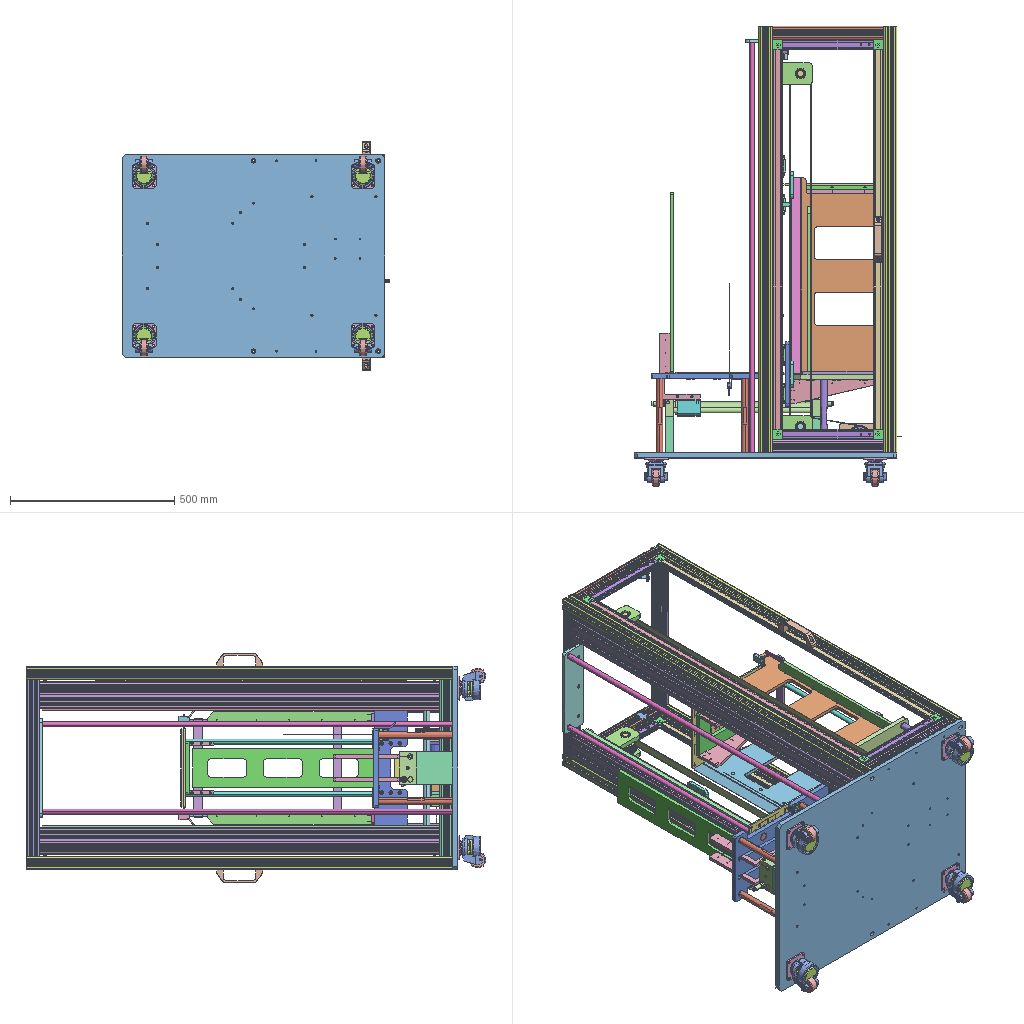Assembly | STEP file | 78 different items | 208 placed | box 815 x 1400 x 700 mm
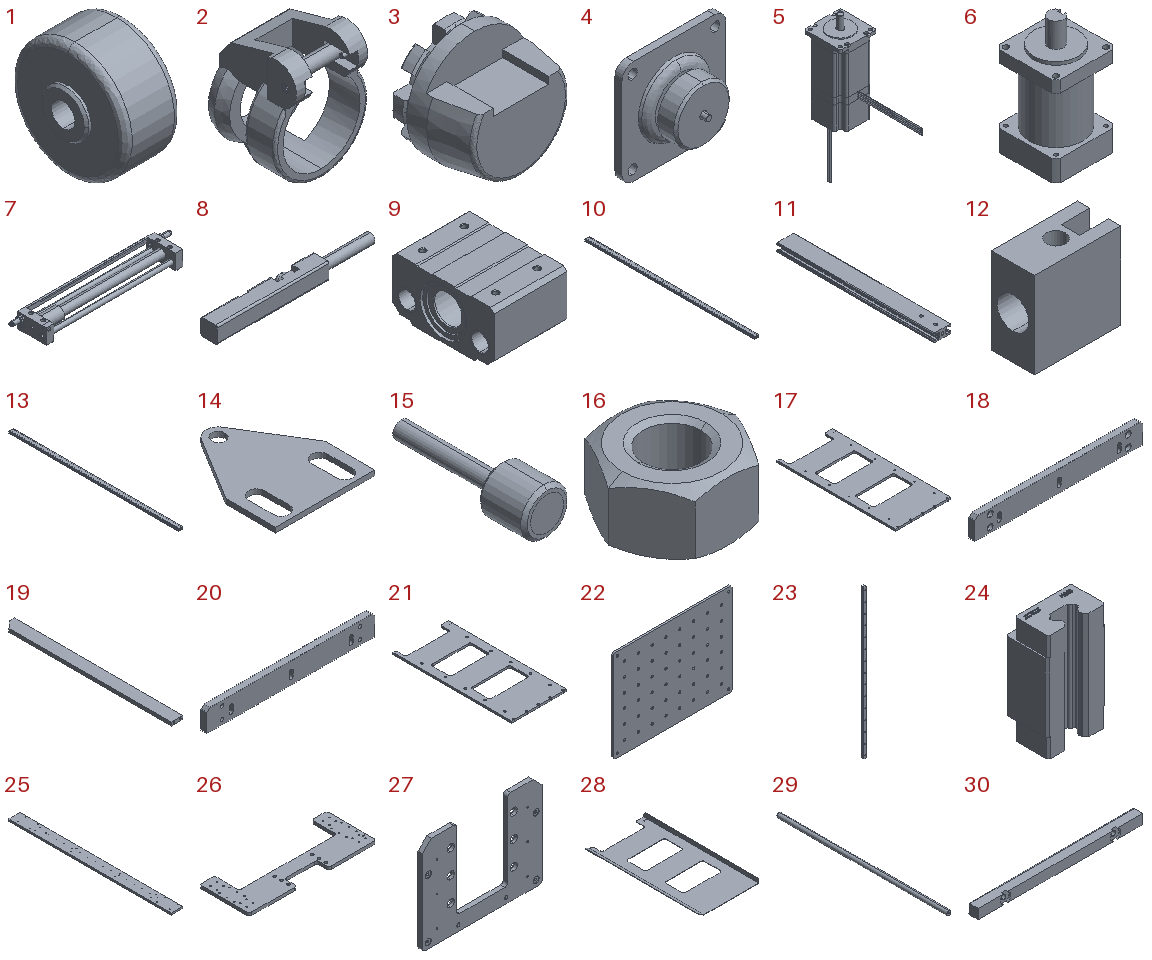Parts list (item | name | quantity | parent item | size | volume):
1 | HI_CGR51-60-U-001 | x4 | in CGR51-60-U, CGR51-60-U-1, CGR51-60-U-2, CGR51-60-U-3 | 28 x 49 x 49 mm | 43678 mm3
2 | HI_CGR51-60-U-002 | x4 | in CGR51-60-U, CGR51-60-U-1, CGR51-60-U-2, CGR51-60-U-3 | 70 x 63 x 89.5 mm | 81661 mm3
3 | HI_CGR51-60-U-004 | x4 | in CGR51-60-U, CGR51-60-U-1, CGR51-60-U-2, CGR51-60-U-3 | 55 x 39.5 x 55 mm | 65698 mm3
4 | HI_CGR51-60-U-003 | x4 | in CGR51-60-U, CGR51-60-U-1, CGR51-60-U-2, CGR51-60-U-3 | 73 x 29.8 x 73 mm | 47628 mm3
5 | Leadshine 57HSB21A (with brake) | x1 | in 57 Leadshine stepper with brake and 2-stage reducer (1:30) assembly | 57.15 x 157.15 x 237 mm | 340795 mm3
6 | 57 stepper reducer, 2-stage, ratio 30 | x1 | in 57 Leadshine stepper with brake and 2-stage reducer (1:30) assembly | 57 x 57 x 110 mm | 202914 mm3
7 | _RMT-25X350-S-A(0)-GN-2_rod | x1 | in RMT25X350SA_0_+_DS1-GN-2_ | 555 x 106.4 x 53 mm | 757073 mm3
8 | _CS1-E | x2 | in RMT25X350SA_0_+_DS1-GN-2_ | 48.8 x 5.2 x 5 mm | 895.745 mm3
9 | _RMT-25X350-S(0)_body | x1 | in RMT25X350SA_0_+_DS1-GN-2_ | 70 x 97 x 52 mm | 215787 mm3
10 | GB1530T-6-30x15x1155-BASHOU | x2 | in 1220x340 door, 1220x340 door-1 | 30 x 1157 x 15 mm | 281206 mm3
11 | GB1530T-6-30x15x275 | x4 | in 1220x340 door, 1220x340 door-1 | 30 x 277 x 15 mm | 67010 mm3
12 | Right-angle connecting block | x8 | in 1220x340 door, 1220x340 door-1 | 30 x 15 x 30 mm | 8895 mm3
13 | GB1530T-6-30x15x1155 | x2 | in 1220x340 door, 1220x340 door-1 | 30 x 1157 x 15 mm | 281619 mm3
14 | Door catch sheet metal | x4 | in Door catch, Door catch-1, Door catch-2, Door catch-3 | 40 x 48 x 2 mm | 2431 mm3
15 | Pedestal magnet | x4 | in Door catch, Door catch-1, Door catch-2, Door catch-3 | 14 x 44 x 14 mm | 2702 mm3
16 | hex nuts, style 1-grades ab gb(GB_FASTENER_NUT_SNAB1 M5-N) | x8 | in Door catch, Door catch-1, Door catch-2, Door catch-3 | 9.238 x 8 x 4.7 mm | 190.603 mm3
17 | PN_0033 | x1 | in Side bracket | 279.996 x 599.997 x 10 mm | 1160926 mm3
18 | PN_0034 | x1 | in Side bracket | 280 x 10 x 35 mm | 92081 mm3
19 | PN_0035 | x4 | in Side bracket | 35 x 500 x 10 mm | 171757 mm3
20 | PN_0037 | x1 | in Side bracket | 280 x 10 x 35 mm | 92081 mm3
21 | PN_0036 | x1 | in Side bracket | 279.996 x 599.997 x 10 mm | 1160926 mm3
22 | Three-part square aluminium plate (2R8, 6R5) | x3 | - | 310 x 4.5 x 240 mm | 298192 mm3
23 | HGR15-rail L870 | x2 | - | 15 x 15 x 870 mm | 160134 mm3
24 | HGH15-slider | x8 | - | 34 x 23.7 x 61.7 mm | 37046 mm3
25 | PN_0029 | x1 | - | 90 x 1255 x 15 mm | 1602482 mm3
26 | PN_0002 | x1 | - | 510 x 200 x 12 mm | 664330 mm3
27 | PN_0003 | x1 | - | 400 x 15 x 315 mm | 1138040 mm3
28 | PN_0004(Default) | x1 | - | 313.731 x 597.76 x 21.5 mm | 225169 mm3
29 | PN_0005 | x2 | - | 15 x 580 x 15 mm | 101796 mm3
30 | PN_0006 | x1 | - | 240 x 15 x 14 mm | 46724 mm3
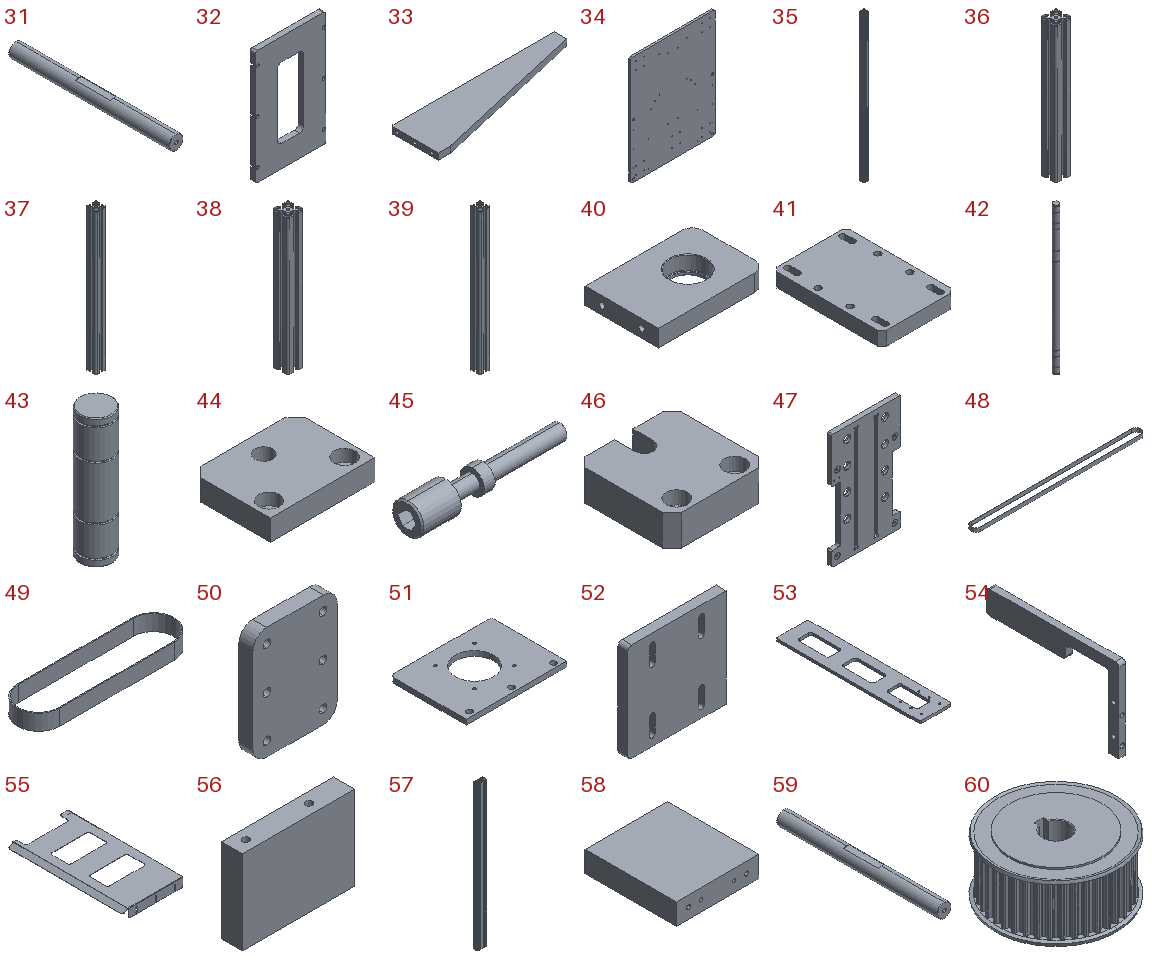31 | PN_0007 | x4 | - | 20 x 228 x 20 mm | 70235 mm3
32 | PN_0008 | x2 | - | 160 x 12 x 260 mm | 379891 mm3
33 | PN_0009 | x4 | - | 260 x 75 x 10 mm | 127129 mm3
34 | PN_0010 | x1 | - | 620 x 15 x 800 mm | 7409131 mm3
35 | HM-8-4040D-L1300 | x4 | - | 40 x 40 x 1300 mm | 890054 mm3
36 | HM-8-4040D-L340-machining required | x2 | - | 40 x 40 x 340 mm | 231664 mm3
37 | HM-8-4040D-L540-machining required | x1 | - | 40 x 40 x 540 mm | 368969 mm3
38 | HM-8-4040D-L340 | x2 | - | 40 x 40 x 340 mm | 232783 mm3
39 | HM-8-4040D-L540 | x2 | - | 40 x 40 x 540 mm | 369715 mm3
40 | PN_0012 | x8 | - | 95 x 65 x 15 mm | 79674 mm3
41 | PN_0013 | x4 | - | 80 x 120 x 15 mm | 132965 mm3
42 | PN_0014 | x1 | - | 20 x 20 x 530 mm | 164764 mm3
43 | PN_0015 | x2 | - | 20 x 20 x 80 mm | 24503 mm3
44 | PN_0016 | x2 | - | 50 x 38 x 10 mm | 17083 mm3
45 | AJKTN10-50 adjusting screw | x2 | - | 99 x 20 x 20 mm | 13265 mm3
46 | PN_0017 | x2 | - | 50 x 50 x 16 mm | 35086 mm3
47 | PN_0018 | x1 | - | 240 x 15 x 400 mm | 1068440 mm3
48 | Timing belt S5M-width 25-length 2350 (C-HTBN2350S5M-250, steel wire core) | x2 | - | 1142 x 66.7 x 25 mm | 88306 mm3
49 | Timing belt S5M-width 25-length 565 (steel wire core) | x1 | - | 249.2 x 66.7 x 25 mm | 21369 mm3
50 | PN_0021 | x4 | - | 60 x 10 x 80 mm | 43843 mm3
51 | PN_0022 | x1 | - | 120 x 90 x 6 mm | 54372 mm3
52 | PN_0023 | x1 | - | 120 x 12 x 120 mm | 163808 mm3
53 | PN_0011 | x1 | - | 120 x 550 x 10 mm | 459826 mm3
54 | PN_0019 | x2 | - | 10 x 200 x 125 mm | 67703 mm3
55 | PN_0024(Default) | x1 | - | 313.731 x 599.997 x 46.5 mm | 244261 mm3
56 | PN_0025 | x1 | - | 80 x 15 x 60 mm | 69644 mm3
57 | HM-8-4080D-L1220 | x2 | - | 80 x 40 x 1220 mm | 1475152 mm3
58 | PN_0020 | x2 | - | 100 x 110 x 25.5 mm | 279122 mm3
59 | PN_0026 | x4 | - | 20 x 230 x 20 mm | 70863 mm3
60 | EBJ52-S5M250-40-A-N-d14 | x1 | - | 67 x 67 x 32 mm | 87087 mm3
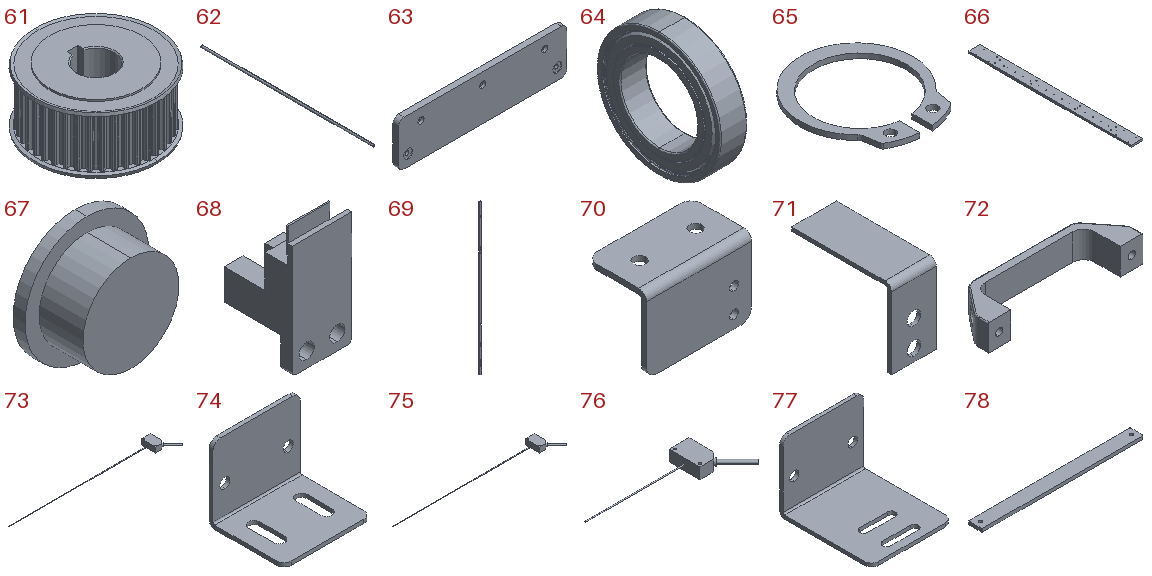61 | EBJ52-S5M250-40-A-N-d20 | x5 | - | 67 x 67 x 32 mm | 81650 mm3
62 | PN_0027 | x2 | - | 16 x 1252 x 16 mm | 251030 mm3
63 | PN_0028 | x1 | - | 300 x 10 x 80 mm | 235858 mm3
64 | BAY6804ZZ lifting mechanism drive bearing | x8 | - | 7 x 32 x 32 mm | 2847 mm3
65 | Shaft retaining ring 20 (GB_CONNECTING_PIECE_RING_RRA 20) | x8 | - | 22.5 x 25.161 x 1 mm | 153.893 mm3
66 | PN_0001 | x1 | - | 90 x 1255 x 15 mm | 1602655 mm3
67 | Universal ball bearing H21xD31xh6-40KG | x14 | - | 31 x 21 x 31 mm | 8224 mm3
68 | xgSENSOR(EE-SX674) | x4 | - | 13.6 x 15.5 x 27.3 mm | 2060 mm3
69 | 9x6 sensor aluminium slot M3 type-L950 | x1 | - | 9 x 6 x 950 mm | 30935 mm3
70 | PN_0030(Default) | x4 | - | 30 x 17.237 x 21.5 mm | 1592 mm3
71 | PN_0031(Default) | x1 | - | 12 x 26.737 x 21 mm | 534.113 mm3
72 | Door handle | x2 | - | 140 x 40 x 24 mm | 37832 mm3
73 | Photoelectric sensor CX421 (NPN, 300mm) | x1 | - | 341.148 x 54.448 x 11.2 mm | 7391 mm3
74 | PN_0038(Default) | x1 | - | 35 x 30 x 30 mm | 2806 mm3
75 | Photoelectric sensor CX411D (NPN, receiver, with slit light shield OS-CX-2)) | x1 | - | 341.148 x 54.448 x 11.2 mm | 7391 mm3
76 | Photoelectric sensor CX411D (NPN, receiver) | x1 | - | 141.148 x 54.448 x 11.2 mm | 7234 mm3
77 | PN_0039(Default) | x2 | - | 35 x 40 x 30 mm | 3359 mm3
78 | PN_0032 | x2 | - | 300 x 25 x 6 mm | 44703 mm3
Placements (level | parent | child | x y z in mm | rotation matrix by rows):
1 | subassembly 2 | CGR51-60-U | -198.5 -701.0 280.0 | 1 0 0 0 1 0 0 0 1
2 | CGR51-60-U | HI_CGR51-60-U-001 | -0.0 -0.0 -0.0 | 1 0 0 0 1 0 0 0 1
2 | CGR51-60-U | HI_CGR51-60-U-002 | -0.0 -0.0 -0.0 | 1 0 0 0 1 0 0 0 1
2 | CGR51-60-U | HI_CGR51-60-U-004 | -0.0 -0.0 -0.0 | 1 0 0 0 1 0 0 0 1
2 | CGR51-60-U | HI_CGR51-60-U-003 | -0.0 4.0 -0.0 | 1 0 0 0 1 0 0 0 1
1 | subassembly 2 | CGR51-60-U-1 | -198.5 -701.0 -280.0 | -1 0 0 0 1 0 0 0 -1
2 | CGR51-60-U-1 | HI_CGR51-60-U-001 | -0.0 -0.0 -0.0 | 1 0 0 0 1 0 0 0 1
2 | CGR51-60-U-1 | HI_CGR51-60-U-002 | -0.0 -0.0 -0.0 | 1 0 0 0 1 0 0 0 1
2 | CGR51-60-U-1 | HI_CGR51-60-U-004 | -0.0 -0.0 -0.0 | 1 0 0 0 1 0 0 0 1
2 | CGR51-60-U-1 | HI_CGR51-60-U-003 | -0.0 4.0 -0.0 | 1 0 0 0 1 0 0 0 1
1 | subassembly 2 | CGR51-60-U-2 | 468.5 -701.0 -280.0 | -1 0 0 0 1 0 0 0 -1
2 | CGR51-60-U-2 | HI_CGR51-60-U-001 | -0.0 -0.0 -0.0 | 1 0 0 0 1 0 0 0 1
2 | CGR51-60-U-2 | HI_CGR51-60-U-002 | -0.0 -0.0 -0.0 | 1 0 0 0 1 0 0 0 1
2 | CGR51-60-U-2 | HI_CGR51-60-U-004 | -0.0 -0.0 -0.0 | 1 0 0 0 1 0 0 0 1
2 | CGR51-60-U-2 | HI_CGR51-60-U-003 | -0.0 4.0 -0.0 | 1 0 0 0 1 0 0 0 1
1 | subassembly 2 | CGR51-60-U-3 | 468.5 -701.0 280.0 | 1 0 0 0 1 0 0 0 1
2 | CGR51-60-U-3 | HI_CGR51-60-U-001 | -0.0 -0.0 -0.0 | 1 0 0 0 1 0 0 0 1
2 | CGR51-60-U-3 | HI_CGR51-60-U-002 | -0.0 -0.0 -0.0 | 1 0 0 0 1 0 0 0 1
2 | CGR51-60-U-3 | HI_CGR51-60-U-004 | -0.0 -0.0 -0.0 | 1 0 0 0 1 0 0 0 1
2 | CGR51-60-U-3 | HI_CGR51-60-U-003 | -0.0 4.0 -0.0 | 1 0 0 0 1 0 0 0 1
1 | subassembly 2 | 57 Leadshine stepper with brake and 2-stage reducer (1:30) assembly | 421.517 -575.0 -72.0 | 0 -1 0 1 0 0 0 0 1
2 | 57 Leadshine stepper with brake and 2-stage reducer (1:30) assembly | Leadshine 57HSB21A (with brake) | -0.0 -0.0 -0.0 | 1 0 0 0 1 0 0 0 1
2 | 57 Leadshine stepper with brake and 2-stage reducer (1:30) assembly | 57 stepper reducer, 2-stage, ratio 30 | -0.0 0.0 90.0 | 1 0 0 0 1 0 0 0 1
1 | subassembly 2 | RMT25X350SA_0_+_DS1-GN-2_ | -171.0 -488.5 -0.0 | 1 0 0 0 0 1 0 -1 -0
2 | RMT25X350SA_0_+_DS1-GN-2_ | _RMT-25X350-S-A(0)-GN-2_rod | -0.0 -0.0 -0.0 | 1 0 0 0 1 0 0 0 1
2 | RMT25X350SA_0_+_DS1-GN-2_ | _CS1-E | 12.0 51.0 17.5 | 1 0 0 0 1 0 0 0 1
2 | RMT25X350SA_0_+_DS1-GN-2_ | _CS1-E | 462.0 51.0 17.5 | -1 0 0 0 1 0 0 0 -1
2 | RMT25X350SA_0_+_DS1-GN-2_ | _RMT-25X350-S(0)_body | 10.0 0.0 -0.0 | 1 0 0 0 1 0 0 0 1
1 | subassembly 2 | 1220x340 door | 703.104 372.073 -1056.974 | 1 0 0 0 1 0 0 0 1
2 | 1220x340 door | GB1530T-6-30x15x1155-BASHOU | -224.604 -925.573 1359.474 | 1 0 0 0 1 0 0 0 1
2 | 1220x340 door | GB1530T-6-30x15x275 | -239.604 246.427 1359.474 | 0 -1 0 1 0 0 0 0 1
2 | 1220x340 door | GB1530T-6-30x15x275 | -239.604 -940.573 1359.474 | 0 -1 0 1 0 0 0 0 1
2 | 1220x340 door | Right-angle connecting block | -224.604 246.427 1366.974 | -1 0 0 0 0 -1 0 -1 -0
2 | 1220x340 door | Right-angle connecting block | -531.604 -940.573 1366.974 | 1 0 0 0 0 1 0 -1 0
2 | 1220x340 door | Right-angle connecting block | -224.604 -940.573 1366.974 | 0 0 -1 1 0 0 0 -1 -0
2 | 1220x340 door | Right-angle connecting block | -531.604 246.427 1366.974 | 0 0 1 -1 0 0 0 -1 -0
2 | 1220x340 door | GB1530T-6-30x15x1155 | -531.604 -925.573 1359.474 | 1 0 0 0 1 0 0 0 1
1 | subassembly 2 | Door catch | 420.014 -588.586 -212.423 | -1 0 0 0 1 0 0 0 -1
2 | Door catch | Door catch sheet metal | -5.737 1.086 47.062 | 1 0 0 0 1 0 0 0 1
2 | Door catch | Pedestal magnet | -5.737 20.086 80.577 | 0.6867 0 0.7269 -0.7269 0 0.6867 0 -1 0
2 | Door catch | hex nuts, style 1-grades ab gb(GB_FASTENER_NUT_SNAB1 M5-N) | -5.737 20.086 53.762 | 0.9973 0.07331 0 -0.07331 0.9973 0 0 0 1
2 | Door catch | hex nuts, style 1-grades ab gb(GB_FASTENER_NUT_SNAB1 M5-N) | -5.737 20.086 47.062 | 1 0 0 0 1 0 0 0 1
1 | subassembly 2 | Door catch-1 | 431.486 638.586 -214.423 | 1 0 0 0 -1 0 0 0 -1
2 | Door catch-1 | Door catch sheet metal | -5.737 1.086 47.062 | 1 0 0 0 1 0 0 0 1
2 | Door catch-1 | Pedestal magnet | -5.737 20.086 80.577 | 0.6867 0 0.7269 -0.7269 0 0.6867 0 -1 0
2 | Door catch-1 | hex nuts, style 1-grades ab gb(GB_FASTENER_NUT_SNAB1 M5-N) | -5.737 20.086 47.062 | 1 0 0 0 1 0 0 0 1
2 | Door catch-1 | hex nuts, style 1-grades ab gb(GB_FASTENER_NUT_SNAB1 M5-N) | -5.737 20.086 53.762 | 0.9973 0.07331 0 -0.07331 0.9973 0 0 0 1
1 | subassembly 2 | 1220x340 door-1 | 703.104 -322.073 1056.974 | 1 0 0 0 -1 0 0 0 -1
2 | 1220x340 door-1 | GB1530T-6-30x15x1155-BASHOU | -224.604 -925.573 1359.474 | 1 0 0 0 1 0 0 0 1
2 | 1220x340 door-1 | GB1530T-6-30x15x275 | -239.604 246.427 1359.474 | 0 -1 0 1 0 0 0 0 1
2 | 1220x340 door-1 | GB1530T-6-30x15x275 | -239.604 -940.573 1359.474 | 0 -1 0 1 0 0 0 0 1
2 | 1220x340 door-1 | Right-angle connecting block | -531.604 -940.573 1366.974 | 1 0 0 0 0 1 0 -1 0
2 | 1220x340 door-1 | Right-angle connecting block | -224.604 -940.573 1366.974 | 0 0 -1 1 0 0 0 -1 -0
2 | 1220x340 door-1 | Right-angle connecting block | -531.604 246.427 1366.974 | 0 0 1 -1 0 0 0 -1 -0
2 | 1220x340 door-1 | Right-angle connecting block | -224.604 246.427 1366.974 | -1 0 0 0 0 -1 0 -1 -0
2 | 1220x340 door-1 | GB1530T-6-30x15x1155 | -531.604 -925.573 1359.474 | 1 0 0 0 1 0 0 0 1
1 | subassembly 2 | Door catch-2 | 420.014 638.586 214.423 | -1 0 0 0 -1 0 0 0 1
2 | Door catch-2 | Door catch sheet metal | -5.737 1.086 47.062 | 1 0 0 0 1 0 0 0 1
2 | Door catch-2 | Pedestal magnet | -5.737 20.086 80.577 | 0.6867 0 0.7269 -0.7269 0 0.6867 0 -1 0
2 | Door catch-2 | hex nuts, style 1-grades ab gb(GB_FASTENER_NUT_SNAB1 M5-N) | -5.737 20.086 53.762 | 0.9973 0.07331 0 -0.07331 0.9973 0 0 0 1
2 | Door catch-2 | hex nuts, style 1-grades ab gb(GB_FASTENER_NUT_SNAB1 M5-N) | -5.737 20.086 47.062 | 1 0 0 0 1 0 0 0 1
1 | subassembly 2 | Door catch-3 | 431.486 -588.586 212.423 | 1 0 0 0 1 0 0 0 1
2 | Door catch-3 | Door catch sheet metal | -5.737 1.086 47.062 | 1 0 0 0 1 0 0 0 1
2 | Door catch-3 | Pedestal magnet | -5.737 20.086 80.577 | 0.6867 0 0.7269 -0.7269 0 0.6867 0 -1 0
2 | Door catch-3 | hex nuts, style 1-grades ab gb(GB_FASTENER_NUT_SNAB1 M5-N) | -5.737 20.086 47.062 | 1 0 0 0 1 0 0 0 1
2 | Door catch-3 | hex nuts, style 1-grades ab gb(GB_FASTENER_NUT_SNAB1 M5-N) | -5.737 20.086 53.762 | 0.9973 0.07331 0 -0.07331 0.9973 0 0 0 1
1 | subassembly 2 | Side bracket | 383.48 -386.0 126.5 | 1 0 0 0 1 0 0 0 1
2 | Side bracket | PN_0033 | -0.0 -0.0 -0.0 | 1 0 0 0 1 0 0 0 1
2 | Side bracket | PN_0034 | -0.287 5.0 27.5 | 1 0 0 0 1 0 0 0 1
2 | Side bracket | PN_0035 | 115.0 260.0 -280.5 | 0 0 -1 0 1 0 1 0 0
2 | Side bracket | PN_0035 | -115.0 260.0 27.5 | 0 0 1 0 1 0 -1 0 0
2 | Side bracket | PN_0035 | 115.0 260.0 27.5 | 0 0 1 0 1 0 -1 0 0
2 | Side bracket | PN_0035 | -115.0 260.0 -280.5 | 0 0 -1 0 1 0 1 0 0
2 | Side bracket | PN_0037 | -0.287 5.0 -280.5 | 1 0 0 0 -1 0 0 0 -1
2 | Side bracket | PN_0036 | -0.0 -0.0 -263.0 | 1 0 0 0 1 0 0 0 1
1 | subassembly 2 | Three-part square aluminium plate (2R8, 6R5) | 16.0 -384.0 -0.0 | 1 0 0 0 1 0 0 0 1
1 | subassembly 2 | Three-part square aluminium plate (2R8, 6R5) | 346.0 190.7 0.0 | 1 0 0 0 1 0 0 0 1
1 | subassembly 2 | Three-part square aluminium plate (2R8, 6R5) | 346.0 -386.0 -0.0 | 1 0 0 0 1 0 0 0 1
1 | subassembly 2 | HGR15-rail L870 | 183.0 -410.0 -225.0 | 0 1 0 0 0 1 1 0 0
1 | subassembly 2 | HGR15-rail L870 | 183.0 -410.0 225.0 | 0 1 0 0 0 1 1 0 0
1 | subassembly 2 | HGH15-slider | 183.0 -326.7 -225.0 | 0 1 0 0 0 1 1 0 0
1 | subassembly 2 | HGH15-slider | 183.0 -445.3 -225.0 | 0 1 0 0 0 1 1 0 0
1 | subassembly 2 | HGH15-slider | 183.0 -326.7 225.0 | 0 1 0 0 0 1 1 0 0
1 | subassembly 2 | HGH15-slider | 183.0 250.0 -225.0 | 0 1 0 0 0 1 1 0 0
1 | subassembly 2 | HGH15-slider | 183.0 131.4 225.0 | 0 1 0 0 0 1 1 0 0
1 | subassembly 2 | HGH15-slider | 183.0 250.0 225.0 | 0 1 0 0 0 1 1 0 0
1 | subassembly 2 | HGH15-slider | 183.0 131.4 -225.0 | 0 1 0 0 0 1 1 0 0
1 | subassembly 2 | HGH15-slider | 183.0 -445.3 225.0 | 0 1 0 0 0 1 1 0 0
1 | subassembly 2 | PN_0029 | 170.0 2.5 0.0 | 0 0 -1 0 1 0 1 0 0
1 | subassembly 2 | PN_0002 | 208.0 -386.0 0.0 | 0 0 -1 0 1 0 1 0 -0
1 | subassembly 2 | PN_0003 | 370.5 -386.0 0.0 | 0 0 -1 0 1 0 1 0 -0
1 | subassembly 2 | PN_0004(Default) | 383.0 -84.883 126.5 | 1 0 0 0 1 0 0 0 1
1 | subassembly 2 | PN_0005 | 509.0 -388.0 80.0 | -0.07973 0 -0.9968 0 1 0 0.9968 0 -0.07973
1 | subassembly 2 | PN_0005 | 509.0 -388.0 -80.0 | -0.07973 0 -0.9968 0 1 0 0.9968 0 -0.07973
1 | subassembly 2 | PN_0006 | 509.0 204.0 0.0 | 0 0 1 0 1 0 -1 0 0
1 | subassembly 2 | PN_0007 | 313.0 -627.0 180.0 | 0 0 -1 0 1 0 1 0 -0
1 | subassembly 2 | PN_0007 | 508.0 -627.0 -180.0 | 0 0 1 0 1 0 -1 0 0
1 | subassembly 2 | PN_0007 | 313.0 -627.0 -180.0 | 0 0 1 0 1 0 -1 0 0
1 | subassembly 2 | PN_0007 | 508.0 -627.0 180.0 | 0 0 1 0 1 0 -1 0 0
1 | subassembly 2 | PN_0008 | 338.0 184.7 0.0 | 0 0 -1 0 1 0 1 0 -0
1 | subassembly 2 | PN_0008 | 338.0 -392.0 0.0 | 0 0 -1 0 1 0 1 0 -0
1 | subassembly 2 | PN_0009 | 208.0 103.7 -75.0 | 1 0 0 0 1 0 0 0 1
1 | subassembly 2 | PN_0009 | 208.0 -473.0 75.0 | 1 0 0 0 1 0 0 0 1
1 | subassembly 2 | PN_0009 | 208.0 -473.0 -75.0 | 1 0 0 0 1 0 0 0 1
1 | subassembly 2 | PN_0009 | 208.0 103.7 75.0 | 1 0 0 0 1 0 0 0 1
1 | subassembly 2 | PN_0010 | 135.0 -640.0 0.0 | 0 0 -1 0 1 0 1 0 0
1 | subassembly 2 | HM-8-4040D-L1300 | -3395.85 25.0 -165.119 | 1 0 0 0 0 -1 0 1 0
1 | subassembly 2 | HM-8-4040D-L1300 | -3015.85 25.0 -165.119 | 1 0 0 0 0 -1 0 1 0
1 | subassembly 2 | HM-8-4040D-L1300 | -3015.85 25.0 -745.119 | 1 0 0 0 0 -1 0 1 0
1 | subassembly 2 | HM-8-4040D-L1300 | -3395.85 25.0 -745.119 | 1 0 0 0 0 -1 0 1 0
1 | subassembly 2 | HM-8-4040D-L340-machining required | 325.0 -1060.119 -3240.85 | 0 0 -1 0 1 0 1 0 0
1 | subassembly 2 | HM-8-4040D-L340-machining required | 325.0 -1060.119 -3820.85 | 0 0 -1 0 1 0 1 0 0
1 | subassembly 2 | HM-8-4040D-L540-machining required | -3395.85 -1060.119 0.0 | 1 0 0 0 1 0 0 0 1
1 | subassembly 2 | HM-8-4040D-L340 | 325.0 199.881 -3240.85 | 0 0 -1 0 1 0 1 0 0
1 | subassembly 2 | HM-8-4040D-L340 | 325.0 199.881 -3820.85 | 0 0 -1 0 1 0 1 0 0
1 | subassembly 2 | HM-8-4040D-L540 | -3395.85 199.881 -0.0 | 1 0 0 0 1 0 0 0 1
1 | subassembly 2 | HM-8-4040D-L540 | -3015.85 199.881 0.0 | 1 0 0 0 1 0 0 0 1
1 | subassembly 2 | PN_0012 | 230.5 530.0 -192.5 | 1 0 0 0 1 0 0 0 1
1 | subassembly 2 | PN_0012 | 230.5 -545.0 -257.5 | 1 0 0 0 -1 0 0 0 -1
1 | subassembly 2 | PN_0012 | 230.5 530.0 -257.5 | 1 0 0 0 -1 0 0 0 -1
1 | subassembly 2 | PN_0012 | 230.5 530.0 257.5 | 1 0 0 0 1 0 0 0 1
1 | subassembly 2 | PN_0012 | 230.5 -545.0 192.5 | 1 0 0 0 -1 0 0 0 -1
1 | subassembly 2 | PN_0012 | 230.5 -545.0 257.5 | 1 0 0 0 1 0 0 0 1
1 | subassembly 2 | PN_0012 | 230.5 -545.0 -192.5 | 1 0 0 0 1 0 0 0 1
1 | subassembly 2 | PN_0012 | 230.5 530.0 192.5 | 1 0 0 0 -1 0 0 0 -1
1 | subassembly 2 | PN_0013 | 175.5 -545.0 -225.0 | 0 0 1 0 1 0 -1 0 0
1 | subassembly 2 | PN_0013 | 175.5 -545.0 225.0 | 0 0 1 0 1 0 -1 0 0
1 | subassembly 2 | PN_0013 | 175.5 530.0 -225.0 | 0 0 1 0 1 0 -1 0 0
1 | subassembly 2 | PN_0013 | 175.5 530.0 225.0 | 0 0 1 0 1 0 -1 0 0
1 | subassembly 2 | PN_0014 | 241.5 -545.0 0.0 | -0.9897 -0.143 0 0.143 -0.9897 0 0 0 1
1 | subassembly 2 | PN_0015 | 241.5 530.0 225.0 | 0.7857 -0.6186 0 0.6186 0.7857 0 0 0 1
1 | subassembly 2 | PN_0015 | 241.5 530.0 -225.0 | 0.7857 -0.6186 0 0.6186 0.7857 0 0 0 1
1 | subassembly 2 | PN_0016 | 187.0 600.0 225.0 | 0 1 0 0 0 1 1 0 -0
1 | subassembly 2 | PN_0016 | 187.0 600.0 -225.0 | 0 1 0 0 0 1 1 0 -0
1 | subassembly 2 | AJKTN10-50 adjusting screw | 196.0 647.0 -225.0 | 0 0.8487 -0.5289 -1 0 0 0 0.5289 0.8487
1 | subassembly 2 | AJKTN10-50 adjusting screw | 196.0 647.0 225.0 | 0 0.8487 -0.5289 -1 0 0 0 0.5289 0.8487
1 | subassembly 2 | PN_0017 | 155.0 646.0 225.0 | 0 1 0 0 0 1 1 0 0
1 | subassembly 2 | PN_0017 | 155.0 646.0 -225.0 | 0 1 0 0 0 1 1 0 0
1 | subassembly 2 | PN_0018 | -13.0 -384.0 -0.0 | 0 0 1 0 1 0 -1 0 0
1 | subassembly 2 | Timing belt S5M-width 25-length 2350 (C-HTBN2350S5M-250, steel wire core) | 241.5 -7.5 225.0 | 0 1 0 -1 0 0 0 0 1
1 | subassembly 2 | Timing belt S5M-width 25-length 2350 (C-HTBN2350S5M-250, steel wire core) | 241.5 -7.5 -225.0 | 0 1 0 -1 0 0 0 0 1
1 | subassembly 2 | Timing belt S5M-width 25-length 565 (steel wire core) | 331.509 -560.0 105.0 | 0.9864 0.1644 0 -0.1644 0.9864 0 0 0 1
1 | subassembly 2 | PN_0021 | 219.65 -386.0 225.0 | 0 1 0 0 0 1 1 0 0
1 | subassembly 2 | PN_0021 | 219.65 -386.0 -225.0 | 0 1 0 0 0 1 1 0 0
1 | subassembly 2 | PN_0021 | 219.65 190.7 -225.0 | 0 1 0 0 0 1 1 0 0
1 | subassembly 2 | PN_0021 | 219.65 190.7 225.0 | 0 1 0 0 0 1 1 0 0
1 | subassembly 2 | PN_0022 | 421.517 -580.0 82.0 | 1 0 0 0 1 0 0 0 1
1 | subassembly 2 | PN_0023 | 421.517 -619.0 22.0 | 0 0 -1 0 1 0 1 0 -0
1 | subassembly 2 | PN_0011 | -149.0 -107.0 -0.0 | 0 0 -1 0 1 0 1 0 0
1 | subassembly 2 | PN_0019 | -126.5 -461.0 35.0 | 0 0 -1 0 1 0 1 0 -0
1 | subassembly 2 | PN_0019 | -126.5 -461.0 -35.0 | 0 0 -1 0 1 0 1 0 -0
1 | subassembly 2 | PN_0024(Default) | 383.0 -84.883 73.5 | 1 0 0 0 1 0 0 0 1
1 | subassembly 2 | PN_0025 | -104.0 -453.5 -0.0 | 1 0 0 0 1 0 0 0 1
1 | subassembly 2 | HM-8-4080D-L1220 | 668.16 635.0 -3562.427 | 0 -1 0 0 0 -1 1 0 0
1 | subassembly 2 | HM-8-4080D-L1220 | 668.16 635.0 -4002.427 | 0 -1 0 0 0 -1 1 0 0
1 | subassembly 2 | PN_0020 | -158.25 -625.0 -0.0 | 0 0 -1 0 1 0 1 0 -0
1 | subassembly 2 | PN_0020 | 290.25 -625.0 -0.0 | 0 0 1 0 1 0 -1 0 0
1 | subassembly 2 | PN_0026 | -188.0 -627.0 -100.0 | 0.464 0 -0.8858 0 1 0 0.8858 0 0.464
1 | subassembly 2 | PN_0026 | 72.0 -627.0 100.0 | 0.9946 0 0.1036 0 1 0 -0.1036 0 0.9946
1 | subassembly 2 | PN_0026 | 72.0 -627.0 -100.0 | 0.464 0 -0.8858 0 1 0 0.8858 0 0.464
1 | subassembly 2 | PN_0026 | -188.0 -627.0 100.0 | 0.9946 0 0.1036 0 1 0 -0.1036 0 0.9946
1 | subassembly 2 | EBJ52-S5M250-40-A-N-d14 | 421.517 -575.0 121.0 | 0.9064 -0.4224 0 0.4224 0.9064 0 0 0 1
1 | subassembly 2 | EBJ52-S5M250-40-A-N-d20 | 241.5 -545.0 -209.0 | 0.9993 0.0364 0 -0.0364 0.9993 0 0 0 1
1 | subassembly 2 | EBJ52-S5M250-40-A-N-d20 | 241.5 -545.0 121.0 | 0.9993 0.0364 0 -0.0364 0.9993 0 0 0 1
1 | subassembly 2 | EBJ52-S5M250-40-A-N-d20 | 241.5 530.0 -209.0 | 0.9993 0.0364 0 -0.0364 0.9993 0 0 0 1
1 | subassembly 2 | EBJ52-S5M250-40-A-N-d20 | 241.5 -545.0 241.0 | 0.9993 0.0364 0 -0.0364 0.9993 0 0 0 1
1 | subassembly 2 | EBJ52-S5M250-40-A-N-d20 | 241.5 530.0 241.0 | 0.9993 0.0364 0 -0.0364 0.9993 0 0 0 1
1 | subassembly 2 | PN_0027 | 95.0 -625.0 -133.0 | -0.1441 0 0.9896 0 1 0 -0.9896 0 -0.1441
1 | subassembly 2 | PN_0027 | 95.0 -625.0 133.0 | 0.524 0 0.8517 0 1 0 -0.8517 0 0.524
1 | subassembly 2 | PN_0028 | 115.0 625.0 0.0 | 0 0 1 0 1 0 -1 0 0
1 | subassembly 2 | BAY6804ZZ lifting mechanism drive bearing | 241.5 530.0 197.0 | 0 -0.04696 0.9989 0 0.9989 0.04696 -1 0 -0
1 | subassembly 2 | BAY6804ZZ lifting mechanism drive bearing | 241.5 530.0 -253.0 | 0 -0.04696 0.9989 0 0.9989 0.04696 -1 0 -0
1 | subassembly 2 | BAY6804ZZ lifting mechanism drive bearing | 241.5 -545.0 197.0 | 0 -0.04696 0.9989 0 0.9989 0.04696 -1 0 -0
1 | subassembly 2 | BAY6804ZZ lifting mechanism drive bearing | 241.5 -545.0 -253.0 | 0 -0.04696 0.9989 0 0.9989 0.04696 -1 0 -0
1 | subassembly 2 | BAY6804ZZ lifting mechanism drive bearing | 241.5 -545.0 -190.0 | 0 -0.04696 0.9989 0 0.9989 0.04696 -1 0 -0
1 | subassembly 2 | BAY6804ZZ lifting mechanism drive bearing | 241.5 530.0 260.0 | 0 0.5975 0.8019 0 0.8019 -0.5975 -1 0 -0
1 | subassembly 2 | BAY6804ZZ lifting mechanism drive bearing | 241.5 530.0 -190.0 | 0 0.5975 0.8019 0 0.8019 -0.5975 -1 0 -0
1 | subassembly 2 | BAY6804ZZ lifting mechanism drive bearing | 241.5 -545.0 260.0 | 0 -0.04696 0.9989 0 0.9989 0.04696 -1 0 -0
1 | subassembly 2 | Shaft retaining ring 20 (GB_CONNECTING_PIECE_RING_RRA 20) | 241.974 -545.473 -190.0 | 0.7065 0.7077 0 0.7077 -0.7065 0 0 0 -1
1 | subassembly 2 | Shaft retaining ring 20 (GB_CONNECTING_PIECE_RING_RRA 20) | 241.757 530.619 -260.0 | 0.9237 0.383 0 -0.383 0.9237 0 0 0 1
1 | subassembly 2 | Shaft retaining ring 20 (GB_CONNECTING_PIECE_RING_RRA 20) | 241.026 530.473 -209.0 | -0.7065 -0.7077 0 -0.7077 0.7065 0 0 0 -1
1 | subassembly 2 | Shaft retaining ring 20 (GB_CONNECTING_PIECE_RING_RRA 20) | 241.757 529.381 -190.0 | 0.9237 0.383 0 0.383 -0.9237 0 0 0 -1
1 | subassembly 2 | Shaft retaining ring 20 (GB_CONNECTING_PIECE_RING_RRA 20) | 241.757 -544.381 -207.9 | 0.9237 0.383 0 -0.383 0.9237 0 0 0 1
1 | subassembly 2 | Shaft retaining ring 20 (GB_CONNECTING_PIECE_RING_RRA 20) | 241.5 530.67 -241.0 | 1 0 0 0 1 0 0 0 1
1 | subassembly 2 | Shaft retaining ring 20 (GB_CONNECTING_PIECE_RING_RRA 20) | 241.973 -544.526 -261.1 | -0.7077 0.7065 0 0.7065 0.7077 0 0 0 -1
1 | subassembly 2 | Shaft retaining ring 20 (GB_CONNECTING_PIECE_RING_RRA 20) | 241.243 -544.381 -242.1 | -0.9237 -0.383 0 -0.383 0.9237 0 0 0 -1
1 | subassembly 2 | PN_0001 | 170.0 2.5 -0.0 | 0 0 -1 0 1 0 1 0 0
1 | subassembly 2 | Universal ball bearing H21xD31xh6-40KG | 353.0 -403.0 -105.0 | 1 0 0 0 1 0 0 0 1
1 | subassembly 2 | Universal ball bearing H21xD31xh6-40KG | 433.0 -403.0 -105.0 | 1 0 0 0 1 0 0 0 1
1 | subassembly 2 | Universal ball bearing H21xD31xh6-40KG | -93.0 -401.0 -65.5 | 1 0 0 0 1 0 0 0 1
1 | subassembly 2 | Universal ball bearing H21xD31xh6-40KG | 273.0 -403.0 -105.0 | 1 0 0 0 1 0 0 0 1
1 | subassembly 2 | Universal ball bearing H21xD31xh6-40KG | -13.0 -401.0 -65.5 | 1 0 0 0 1 0 0 0 1
1 | subassembly 2 | Universal ball bearing H21xD31xh6-40KG | 67.0 -401.0 -65.5 | 1 0 0 0 1 0 0 0 1
1 | subassembly 2 | Universal ball bearing H21xD31xh6-40KG | 147.0 -401.0 -65.5 | 1 0 0 0 1 0 0 0 1
1 | subassembly 2 | Universal ball bearing H21xD31xh6-40KG | 273.0 -403.0 105.0 | 1 0 0 0 1 0 0 0 1
1 | subassembly 2 | Universal ball bearing H21xD31xh6-40KG | 353.0 -403.0 105.0 | 1 0 0 0 1 0 0 0 1
1 | subassembly 2 | Universal ball bearing H21xD31xh6-40KG | 433.0 -403.0 105.0 | 1 0 0 0 1 0 0 0 1
1 | subassembly 2 | Universal ball bearing H21xD31xh6-40KG | -93.0 -401.0 65.5 | 1 0 0 0 1 0 0 0 1
1 | subassembly 2 | Universal ball bearing H21xD31xh6-40KG | -13.0 -401.0 65.5 | 1 0 0 0 1 0 0 0 1
1 | subassembly 2 | Universal ball bearing H21xD31xh6-40KG | 67.0 -401.0 65.5 | 1 0 0 0 1 0 0 0 1
1 | subassembly 2 | Universal ball bearing H21xD31xh6-40KG | 147.0 -401.0 65.5 | 1 0 0 0 1 0 0 0 1
1 | subassembly 2 | xgSENSOR(EE-SX674) | 174.5 -440.747 258.2 | 0 1 0 0 0 -1 -1 0 0
1 | subassembly 2 | xgSENSOR(EE-SX674) | 174.5 237.812 258.2 | 0 1 0 0 0 -1 -1 0 0
1 | subassembly 2 | xgSENSOR(EE-SX674) | 174.5 -217.244 258.2 | 0 1 0 0 0 -1 -1 0 0
1 | subassembly 2 | xgSENSOR(EE-SX674) | 174.5 205.088 258.2 | 0 1 0 0 0 -1 -1 0 0
1 | subassembly 2 | 9x6 sensor aluminium slot M3 type-L950 | 165.5 -10.0 265.0 | 1 0 0 0 0 -1 0 1 0
1 | subassembly 2 | PN_0030(Default) | 172.263 -432.747 272.5 | 0 -1 0 1 0 0 0 0 1
1 | subassembly 2 | PN_0030(Default) | 172.263 213.088 272.5 | 0 -1 0 1 0 0 0 0 1
1 | subassembly 2 | PN_0030(Default) | 172.263 245.812 272.5 | 0 -1 0 1 0 0 0 0 1
1 | subassembly 2 | PN_0030(Default) | 172.263 -209.244 272.5 | 0 -1 0 1 0 0 0 0 1
1 | subassembly 2 | PN_0031(Default) | 207.263 131.7 258.7 | 0 -1 0 1 0 0 0 0 1
1 | subassembly 2 | Door handle | 478.5 25.0 330.0 | 0 0 -1 -1 0 0 0 1 -0
1 | subassembly 2 | Door handle | 478.5 25.0 -330.0 | 0 0 1 -1 0 0 0 -1 -0
1 | subassembly 2 | Photoelectric sensor CX421 (NPN, 300mm) | 24.4 -419.5 102.5 | 0 0 1 -1 0 0 0 -1 0
1 | subassembly 2 | PN_0038(Default) | 45.0 -400.5 102.5 | 0 -1 0 0 0 -1 1 0 0
1 | subassembly 2 | Photoelectric sensor CX411D (NPN, receiver, with slit light shield OS-CX-2)) | 477.88 193.997 -147.0 | 0 0 1 0 1 0 -1 0 0
1 | subassembly 2 | Photoelectric sensor CX411D (NPN, receiver) | 477.88 193.997 147.0 | 0 0 -1 0 1 0 1 0 -0
1 | subassembly 2 | PN_0039(Default) | 503.48 193.997 128.0 | 0 -1 0 1 0 0 0 0 1
1 | subassembly 2 | PN_0039(Default) | 503.48 193.997 -128.0 | 0 -1 0 -1 0 0 0 0 -1
1 | subassembly 2 | PN_0032 | 528.0 151.497 -0.0 | 0 0 1 0 1 0 -1 0 -0
1 | subassembly 2 | PN_0032 | 534.0 -273.5 -0.0 | 0 0 -1 0 1 0 1 0 0